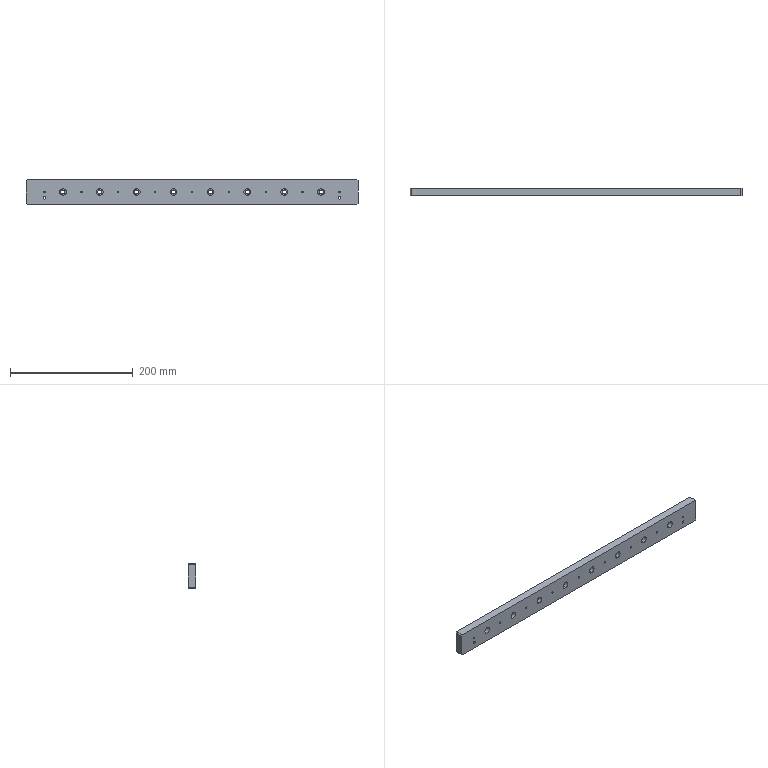Part | SolidWorks | features HoleWzd 3, LPattern 2, Chamfer 1, Extrusion 1 | 1 solid | 90 faces | box 540 x 12 x 40 mm | volume 251867 mm3 | cylinder 54 | cone 18 | plane 18 | commonest cylinder face diameters 2.5 x18 6.6 x16 11 x16 4 x4